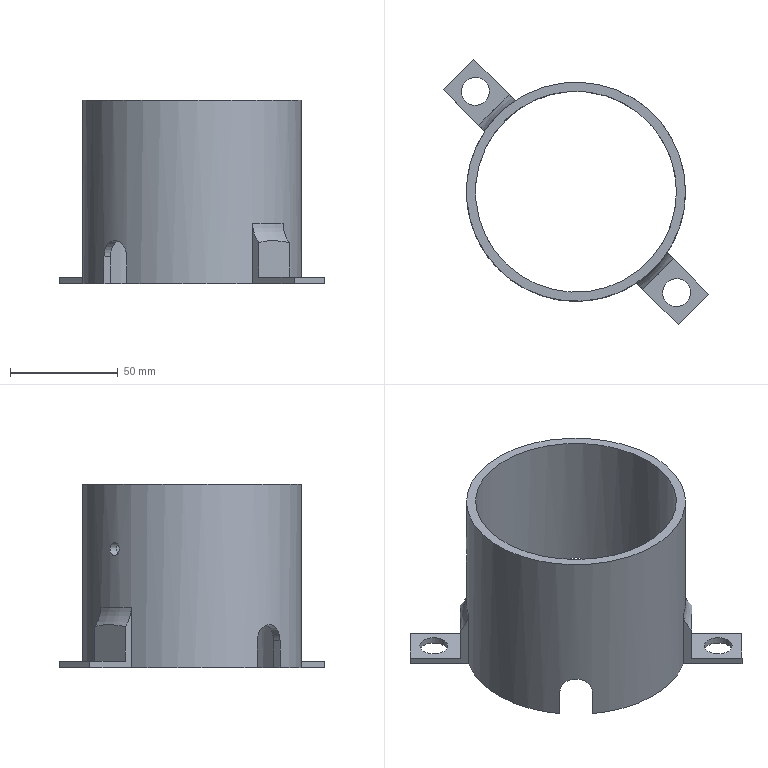Part | NX | features solid 2 | 1 solid | 26 faces | box 123.037 x 123.037 x 85 mm | volume 111745 mm3 | plane 17 | cylinder 7 | torus 2 | commonest cylinder face diameters 13 x2 15 x2 6 x1 93.2 x1 101.6 x1
STEP:
#1=CARTESIAN_POINT('',(-1552.073,-647.927,-105.));
#2=VERTEX_POINT('',#1);
#3=CARTESIAN_POINT('',(-1556.669,-643.331,-105.));
#4=DIRECTION('',(0.,0.,1.));
#5=DIRECTION('',(0.7071,-0.7071,0.));
#6=AXIS2_PLACEMENT_3D('',#3,#4,#5);
#7=CIRCLE('',#6,6.5);
#8=EDGE_CURVE('',#2,#2,#7,.T.);
#9=ORIENTED_EDGE('',*,*,#8,.T.);
#10=EDGE_LOOP('',(#9));
#11=FACE_BOUND('',#10,.T.);
#12=CARTESIAN_POINT('',(-1479.776,-649.169,-105.));
#13=VERTEX_POINT('',#12);
#14=CARTESIAN_POINT('',(-1538.147,-647.711,-105.));
#15=VERTEX_POINT('',#14);
#16=CARTESIAN_POINT('',(-1510.,-690.,-105.));
#17=DIRECTION('',(0.,0.,1.));
#18=DIRECTION('',(0.7071,-0.7071,0.));
#19=AXIS2_PLACEMENT_3D('',#16,#17,#18);
#20=CIRCLE('',#19,50.8);
#21=EDGE_CURVE('',#13,#15,#20,.T.);
#22=ORIENTED_EDGE('',*,*,#21,.F.);
#23=CARTESIAN_POINT('',(-1482.782,-652.175,-105.));
#24=VERTEX_POINT('',#23);
#25=CARTESIAN_POINT('',(-1515.303,-684.697,-105.));
#26=DIRECTION('',(-0.7071,-0.7071,0.));
#27=VECTOR('',#26,1000.);
#28=LINE('',#25,#27);
#29=EDGE_CURVE('',#13,#24,#28,.T.);
#30=ORIENTED_EDGE('',*,*,#29,.T.);
#31=CARTESIAN_POINT('',(-1547.825,-717.218,-105.));
#32=VERTEX_POINT('',#31);
#33=CARTESIAN_POINT('',(-1510.,-690.,-105.));
#34=DIRECTION('',(0.,0.,1.));
#35=DIRECTION('',(0.7071,-0.7071,0.));
#36=AXIS2_PLACEMENT_3D('',#33,#34,#35);
#37=CIRCLE('',#36,46.6);
#38=EDGE_CURVE('',#24,#32,#37,.T.);
#39=ORIENTED_EDGE('',*,*,#38,.T.);
#40=CARTESIAN_POINT('',(-1550.831,-720.224,-105.));
#41=VERTEX_POINT('',#40);
#42=CARTESIAN_POINT('',(-1515.303,-684.697,-105.));
#43=DIRECTION('',(-0.7071,-0.7071,0.));
#44=VECTOR('',#43,1000.);
#45=LINE('',#42,#44);
#46=EDGE_CURVE('',#32,#41,#45,.T.);
#47=ORIENTED_EDGE('',*,*,#46,.T.);
#48=CARTESIAN_POINT('',(-1552.289,-661.853,-105.));
#49=VERTEX_POINT('',#48);
#50=CARTESIAN_POINT('',(-1510.,-690.,-105.));
#51=DIRECTION('',(0.,0.,1.));
#52=DIRECTION('',(0.7071,-0.7071,0.));
#53=AXIS2_PLACEMENT_3D('',#50,#51,#52);
#54=CIRCLE('',#53,50.8);
#55=EDGE_CURVE('',#49,#41,#54,.T.);
#56=ORIENTED_EDGE('',*,*,#55,.F.);
#57=CARTESIAN_POINT('',(-1571.518,-642.624,-105.));
#58=VERTEX_POINT('',#57);
#59=CARTESIAN_POINT('',(-1561.619,-652.523,-105.));
#60=DIRECTION('',(0.7071,-0.7071,0.));
#61=VECTOR('',#60,1000.);
#62=LINE('',#59,#61);
#63=EDGE_CURVE('',#58,#49,#62,.T.);
#64=ORIENTED_EDGE('',*,*,#63,.F.);
#65=CARTESIAN_POINT('',(-1557.376,-628.482,-105.));
#66=VERTEX_POINT('',#65);
#67=CARTESIAN_POINT('',(-1571.518,-642.624,-105.));
#68=DIRECTION('',(0.7071,0.7071,0.));
#69=VECTOR('',#68,1000.);
#70=LINE('',#67,#69);
#71=EDGE_CURVE('',#58,#66,#70,.T.);
#72=ORIENTED_EDGE('',*,*,#71,.T.);
#73=CARTESIAN_POINT('',(-1541.113,-644.745,-105.));
#74=DIRECTION('',(-0.7071,0.7071,0.));
#75=VECTOR('',#74,1000.);
#76=LINE('',#73,#75);
#77=EDGE_CURVE('',#15,#66,#76,.T.);
#78=ORIENTED_EDGE('',*,*,#77,.F.);
#79=EDGE_LOOP('',(#22,#30,#39,#47,#56,#64,#72,#78));
#80=FACE_BOUND('',#79,.T.);
#81=CARTESIAN_POINT('',(-1510.,-690.,-105.));
#82=DIRECTION('',(0.,0.,1.));
#83=DIRECTION('',(0.7071,-0.7071,0.));
#84=AXIS2_PLACEMENT_3D('',#81,#82,#83);
#85=PLANE('',#84);
#86=ADVANCED_FACE('',(#11,#80),#85,.F.);
#87=CARTESIAN_POINT('',(-1546.112,-654.271,-52.988));
#88=VERTEX_POINT('',#87);
#89=CARTESIAN_POINT('',(-1547.688,-655.926,-52.127));
#90=CARTESIAN_POINT('',(-1546.147,-654.276,-53.312));
#91=CARTESIAN_POINT('',(-1544.392,-652.596,-52.552));
#92=CARTESIAN_POINT('',(-1543.503,-651.816,-50.302));
#93=CARTESIAN_POINT('',(-1544.075,-652.313,-47.871));
#94=CARTESIAN_POINT('',(-1545.724,-653.852,-46.689));
#95=CARTESIAN_POINT('',(-1547.402,-655.605,-47.445));
#96=CARTESIAN_POINT('',(-1548.185,-656.498,-49.697));
#97=CARTESIAN_POINT('',(-1547.688,-655.926,-52.127));
#98=CARTESIAN_POINT('',(-1546.147,-654.276,-53.312));
#99=CARTESIAN_POINT('',(-1544.392,-652.596,-52.552));
#100=B_SPLINE_CURVE_WITH_KNOTS('',3,(#89,#90,#91,#92,#93,#94,#95,#96,#97,#98,#99),.UNSPECIFIED.,.T.,.F.,(1,1,1,1,1,1,1,1,1,1,1,1,1,1,1),(-0.007035,-0.00469,-0.002345,0.,0.002345,0.00469,0.007035,0.00938,0.01173,0.01407,0.01642,0.01876,0.02111,0.02345,0.0258),.UNSPECIFIED.);
#101=EDGE_CURVE('',#88,#88,#100,.T.);
#102=ORIENTED_EDGE('',*,*,#101,.T.);
#103=EDGE_LOOP('',(#102));
#104=FACE_BOUND('',#103,.T.);
#105=CARTESIAN_POINT('',(-1459.2,-690.,-20.));
#106=VERTEX_POINT('',#105);
#107=CARTESIAN_POINT('',(-1510.,-690.,-20.));
#108=DIRECTION('',(0.,0.,1.));
#109=DIRECTION('',(1.,0.,0.));
#110=AXIS2_PLACEMENT_3D('',#107,#108,#109);
#111=CIRCLE('',#110,50.8);
#112=EDGE_CURVE('',#106,#106,#111,.T.);
#113=ORIENTED_EDGE('',*,*,#112,.F.);
#114=EDGE_LOOP('',(#113));
#115=FACE_BOUND('',#114,.T.);
#116=CARTESIAN_POINT('',(-1469.169,-659.776,-92.5));
#117=VERTEX_POINT('',#116);
#118=CARTESIAN_POINT('',(-1479.776,-649.169,-92.5));
#119=VERTEX_POINT('',#118);
#120=CARTESIAN_POINT('',(-1469.169,-659.776,-92.5));
#121=CARTESIAN_POINT('',(-1469.169,-659.776,-90.54));
#122=CARTESIAN_POINT('',(-1470.113,-658.437,-86.63));
#123=CARTESIAN_POINT('',(-1473.989,-653.973,-84.184));
#124=CARTESIAN_POINT('',(-1478.43,-650.12,-86.635));
#125=CARTESIAN_POINT('',(-1479.776,-649.169,-90.52));
#126=CARTESIAN_POINT('',(-1479.776,-649.169,-92.5));
#127=B_SPLINE_CURVE_WITH_KNOTS('',3,(#120,#121,#122,#123,#124,#125,#126),.UNSPECIFIED.,.F.,.F.,(4,1,1,1,4),(0.03594,0.04181,0.04767,0.05354,0.05941),.UNSPECIFIED.);
#128=EDGE_CURVE('',#117,#119,#127,.T.);
#129=ORIENTED_EDGE('',*,*,#128,.T.);
#130=CARTESIAN_POINT('',(-1479.776,-649.169,5.));
#131=DIRECTION('',(0.,0.,-1.));
#132=VECTOR('',#131,1000.);
#133=LINE('',#130,#132);
#134=EDGE_CURVE('',#119,#13,#133,.T.);
#135=ORIENTED_EDGE('',*,*,#134,.T.);
#136=ORIENTED_EDGE('',*,*,#21,.T.);
#137=CARTESIAN_POINT('',(-1538.147,-647.711,-77.));
#138=VERTEX_POINT('',#137);
#139=CARTESIAN_POINT('',(-1538.147,-647.711,5.));
#140=DIRECTION('',(0.,0.,-1.));
#141=VECTOR('',#140,1000.);
#142=LINE('',#139,#141);
#143=EDGE_CURVE('',#138,#15,#142,.T.);
#144=ORIENTED_EDGE('',*,*,#143,.F.);
#145=CARTESIAN_POINT('',(-1552.289,-661.853,-77.));
#146=VERTEX_POINT('',#145);
#147=CARTESIAN_POINT('',(-1510.,-690.,-77.));
#148=DIRECTION('',(0.,0.,-1.));
#149=DIRECTION('',(-0.7071,0.7071,0.));
#150=AXIS2_PLACEMENT_3D('',#147,#148,#149);
#151=CIRCLE('',#150,50.8);
#152=EDGE_CURVE('',#138,#146,#151,.F.);
#153=ORIENTED_EDGE('',*,*,#152,.T.);
#154=CARTESIAN_POINT('',(-1552.289,-661.853,-105.));
#155=DIRECTION('',(0.,0.,-1.));
#156=VECTOR('',#155,1000.);
#157=LINE('',#154,#156);
#158=EDGE_CURVE('',#49,#146,#157,.F.);
#159=ORIENTED_EDGE('',*,*,#158,.F.);
#160=ORIENTED_EDGE('',*,*,#55,.T.);
#161=CARTESIAN_POINT('',(-1550.831,-720.224,-92.5));
#162=VERTEX_POINT('',#161);
#163=CARTESIAN_POINT('',(-1550.831,-720.224,5.));
#164=DIRECTION('',(0.,0.,-1.));
#165=VECTOR('',#164,1000.);
#166=LINE('',#163,#165);
#167=EDGE_CURVE('',#41,#162,#166,.F.);
#168=ORIENTED_EDGE('',*,*,#167,.T.);
#169=CARTESIAN_POINT('',(-1540.224,-730.831,-92.5));
#170=VERTEX_POINT('',#169);
#171=CARTESIAN_POINT('',(-1550.831,-720.224,-92.5));
#172=CARTESIAN_POINT('',(-1550.831,-720.224,-90.517));
#173=CARTESIAN_POINT('',(-1549.882,-721.568,-86.634));
#174=CARTESIAN_POINT('',(-1546.014,-726.024,-84.184));
#175=CARTESIAN_POINT('',(-1541.566,-729.884,-86.631));
#176=CARTESIAN_POINT('',(-1540.224,-730.831,-90.541));
#177=CARTESIAN_POINT('',(-1540.224,-730.831,-92.5));
#178=B_SPLINE_CURVE_WITH_KNOTS('',3,(#171,#172,#173,#174,#175,#176,#177),.UNSPECIFIED.,.F.,.F.,(4,1,1,1,4),(0.03522,0.04109,0.04696,0.05283,0.0587),.UNSPECIFIED.);
#179=EDGE_CURVE('',#162,#170,#178,.T.);
#180=ORIENTED_EDGE('',*,*,#179,.T.);
#181=CARTESIAN_POINT('',(-1540.224,-730.831,-105.));
#182=VERTEX_POINT('',#181);
#183=CARTESIAN_POINT('',(-1540.224,-730.831,5.));
#184=DIRECTION('',(0.,0.,-1.));
#185=VECTOR('',#184,1000.);
#186=LINE('',#183,#185);
#187=EDGE_CURVE('',#170,#182,#186,.T.);
#188=ORIENTED_EDGE('',*,*,#187,.T.);
#189=CARTESIAN_POINT('',(-1481.853,-732.289,-105.));
#190=VERTEX_POINT('',#189);
#191=CARTESIAN_POINT('',(-1510.,-690.,-105.));
#192=DIRECTION('',(0.,0.,1.));
#193=DIRECTION('',(0.7071,-0.7071,0.));
#194=AXIS2_PLACEMENT_3D('',#191,#192,#193);
#195=CIRCLE('',#194,50.8);
#196=EDGE_CURVE('',#182,#190,#195,.T.);
#197=ORIENTED_EDGE('',*,*,#196,.T.);
#198=CARTESIAN_POINT('',(-1481.853,-732.289,-77.));
#199=VERTEX_POINT('',#198);
#200=CARTESIAN_POINT('',(-1481.853,-732.289,5.));
#201=DIRECTION('',(0.,0.,-1.));
#202=VECTOR('',#201,1000.);
#203=LINE('',#200,#202);
#204=EDGE_CURVE('',#199,#190,#203,.T.);
#205=ORIENTED_EDGE('',*,*,#204,.F.);
#206=CARTESIAN_POINT('',(-1467.711,-718.147,-77.));
#207=VERTEX_POINT('',#206);
#208=CARTESIAN_POINT('',(-1510.,-690.,-77.));
#209=DIRECTION('',(0.,0.,-1.));
#210=DIRECTION('',(-0.7071,0.7071,0.));
#211=AXIS2_PLACEMENT_3D('',#208,#209,#210);
#212=CIRCLE('',#211,50.8);
#213=EDGE_CURVE('',#199,#207,#212,.F.);
#214=ORIENTED_EDGE('',*,*,#213,.T.);
#215=CARTESIAN_POINT('',(-1467.711,-718.147,-105.));
#216=VERTEX_POINT('',#215);
#217=CARTESIAN_POINT('',(-1467.711,-718.147,-105.));
#218=DIRECTION('',(0.,0.,-1.));
#219=VECTOR('',#218,1000.);
#220=LINE('',#217,#219);
#221=EDGE_CURVE('',#216,#207,#220,.F.);
#222=ORIENTED_EDGE('',*,*,#221,.F.);
#223=CARTESIAN_POINT('',(-1469.169,-659.776,-105.));
#224=VERTEX_POINT('',#223);
#225=CARTESIAN_POINT('',(-1510.,-690.,-105.));
#226=DIRECTION('',(0.,0.,1.));
#227=DIRECTION('',(0.7071,-0.7071,0.));
#228=AXIS2_PLACEMENT_3D('',#225,#226,#227);
#229=CIRCLE('',#228,50.8);
#230=EDGE_CURVE('',#216,#224,#229,.T.);
#231=ORIENTED_EDGE('',*,*,#230,.T.);
#232=CARTESIAN_POINT('',(-1469.169,-659.776,5.));
#233=DIRECTION('',(0.,0.,-1.));
#234=VECTOR('',#233,1000.);
#235=LINE('',#232,#234);
#236=EDGE_CURVE('',#224,#117,#235,.F.);
#237=ORIENTED_EDGE('',*,*,#236,.T.);
#238=EDGE_LOOP('',(#129,#135,#136,#144,#153,#159,#160,#168,#180,#188,#197,#205,#214,#222,#231,#237));
#239=FACE_BOUND('',#238,.T.);
#240=CARTESIAN_POINT('',(-1510.,-690.,5.));
#241=DIRECTION('',(0.,0.,-1.));
#242=DIRECTION('',(-0.7071,0.7071,0.));
#243=AXIS2_PLACEMENT_3D('',#240,#241,#242);
#244=CYLINDRICAL_SURFACE('',#243,50.8);
#245=ADVANCED_FACE('',(#104,#115,#239),#244,.T.);
#246=CARTESIAN_POINT('',(-1482.782,-652.175,-92.5));
#247=VERTEX_POINT('',#246);
#248=CARTESIAN_POINT('',(-1482.782,-652.175,5.));
#249=DIRECTION('',(0.,0.,-1.));
#250=VECTOR('',#249,1000.);
#251=LINE('',#248,#250);
#252=EDGE_CURVE('',#247,#24,#251,.T.);
#253=ORIENTED_EDGE('',*,*,#252,.F.);
#254=CARTESIAN_POINT('',(-1472.175,-662.782,-92.5));
#255=VERTEX_POINT('',#254);
#256=CARTESIAN_POINT('',(-1472.175,-662.782,-92.5));
#257=CARTESIAN_POINT('',(-1472.175,-662.782,-90.515));
#258=CARTESIAN_POINT('',(-1473.108,-661.416,-86.635));
#259=CARTESIAN_POINT('',(-1476.936,-656.948,-84.184));
#260=CARTESIAN_POINT('',(-1481.415,-653.108,-86.63));
#261=CARTESIAN_POINT('',(-1482.782,-652.175,-90.515));
#262=CARTESIAN_POINT('',(-1482.782,-652.175,-92.5));
#263=B_SPLINE_CURVE_WITH_KNOTS('',3,(#256,#257,#258,#259,#260,#261,#262),.UNSPECIFIED.,.F.,.F.,(4,1,1,1,4),(0.,0.00587,0.01174,0.01761,0.02348),.UNSPECIFIED.);
#264=EDGE_CURVE('',#255,#247,#263,.T.);
#265=ORIENTED_EDGE('',*,*,#264,.F.);
#266=CARTESIAN_POINT('',(-1472.175,-662.782,-105.));
#267=VERTEX_POINT('',#266);
#268=CARTESIAN_POINT('',(-1472.175,-662.782,5.));
#269=DIRECTION('',(0.,0.,-1.));
#270=VECTOR('',#269,1000.);
#271=LINE('',#268,#270);
#272=EDGE_CURVE('',#267,#255,#271,.F.);
#273=ORIENTED_EDGE('',*,*,#272,.F.);
#274=CARTESIAN_POINT('',(-1537.218,-727.825,-105.));
#275=VERTEX_POINT('',#274);
#276=CARTESIAN_POINT('',(-1510.,-690.,-105.));
#277=DIRECTION('',(0.,0.,1.));
#278=DIRECTION('',(0.7071,-0.7071,0.));
#279=AXIS2_PLACEMENT_3D('',#276,#277,#278);
#280=CIRCLE('',#279,46.6);
#281=EDGE_CURVE('',#275,#267,#280,.T.);
#282=ORIENTED_EDGE('',*,*,#281,.F.);
#283=CARTESIAN_POINT('',(-1537.218,-727.825,-92.5));
#284=VERTEX_POINT('',#283);
#285=CARTESIAN_POINT('',(-1537.218,-727.825,5.));
#286=DIRECTION('',(0.,0.,-1.));
#287=VECTOR('',#286,1000.);
#288=LINE('',#285,#287);
#289=EDGE_CURVE('',#284,#275,#288,.T.);
#290=ORIENTED_EDGE('',*,*,#289,.F.);
#291=CARTESIAN_POINT('',(-1547.825,-717.218,-92.5));
#292=VERTEX_POINT('',#291);
#293=CARTESIAN_POINT('',(-1547.825,-717.218,-92.5));
#294=CARTESIAN_POINT('',(-1547.825,-717.218,-90.518));
#295=CARTESIAN_POINT('',(-1546.895,-718.58,-86.634));
#296=CARTESIAN_POINT('',(-1543.053,-723.063,-84.183));
#297=CARTESIAN_POINT('',(-1538.578,-726.896,-86.632));
#298=CARTESIAN_POINT('',(-1537.218,-727.825,-90.54));
#299=CARTESIAN_POINT('',(-1537.218,-727.825,-92.5));
#300=B_SPLINE_CURVE_WITH_KNOTS('',3,(#293,#294,#295,#296,#297,#298,#299),.UNSPECIFIED.,.F.,.F.,(4,1,1,1,4),(0.03523,0.0411,0.04697,0.05284,0.05871),.UNSPECIFIED.);
#301=EDGE_CURVE('',#292,#284,#300,.T.);
#302=ORIENTED_EDGE('',*,*,#301,.F.);
#303=CARTESIAN_POINT('',(-1547.825,-717.218,5.));
#304=DIRECTION('',(0.,0.,-1.));
#305=VECTOR('',#304,1000.);
#306=LINE('',#303,#305);
#307=EDGE_CURVE('',#32,#292,#306,.F.);
#308=ORIENTED_EDGE('',*,*,#307,.F.);
#309=ORIENTED_EDGE('',*,*,#38,.F.);
#310=EDGE_LOOP('',(#253,#265,#273,#282,#290,#302,#308,#309));
#311=FACE_BOUND('',#310,.T.);
#312=CARTESIAN_POINT('',(-1543.146,-657.245,-52.987));
#313=VERTEX_POINT('',#312);
#314=CARTESIAN_POINT('',(-1544.717,-658.902,-52.122));
#315=CARTESIAN_POINT('',(-1543.184,-657.249,-53.311));
#316=CARTESIAN_POINT('',(-1541.424,-655.571,-52.556));
#317=CARTESIAN_POINT('',(-1540.526,-654.793,-50.309));
#318=CARTESIAN_POINT('',(-1541.098,-655.283,-47.876));
#319=CARTESIAN_POINT('',(-1542.751,-656.816,-46.69));
#320=CARTESIAN_POINT('',(-1544.427,-658.574,-47.441));
#321=CARTESIAN_POINT('',(-1545.207,-659.474,-49.69));
#322=CARTESIAN_POINT('',(-1544.717,-658.902,-52.122));
#323=CARTESIAN_POINT('',(-1543.184,-657.249,-53.311));
#324=CARTESIAN_POINT('',(-1541.424,-655.571,-52.556));
#325=B_SPLINE_CURVE_WITH_KNOTS('',3,(#314,#315,#316,#317,#318,#319,#320,#321,#322,#323,#324),.UNSPECIFIED.,.T.,.F.,(1,1,1,1,1,1,1,1,1,1,1,1,1,1,1),(-0.007036,-0.00469,-0.002345,0.,0.002345,0.00469,0.007036,0.009381,0.01173,0.01407,0.01642,0.01876,0.02111,0.02345,0.0258),.UNSPECIFIED.);
#326=EDGE_CURVE('',#313,#313,#325,.T.);
#327=ORIENTED_EDGE('',*,*,#326,.F.);
#328=EDGE_LOOP('',(#327));
#329=FACE_BOUND('',#328,.T.);
#330=CARTESIAN_POINT('',(-1463.4,-690.,-20.));
#331=VERTEX_POINT('',#330);
#332=CARTESIAN_POINT('',(-1510.,-690.,-20.));
#333=DIRECTION('',(0.,0.,1.));
#334=DIRECTION('',(1.,0.,0.));
#335=AXIS2_PLACEMENT_3D('',#332,#333,#334);
#336=CIRCLE('',#335,46.6);
#337=EDGE_CURVE('',#331,#331,#336,.T.);
#338=ORIENTED_EDGE('',*,*,#337,.T.);
#339=EDGE_LOOP('',(#338));
#340=FACE_BOUND('',#339,.T.);
#341=CARTESIAN_POINT('',(-1510.,-690.,5.));
#342=DIRECTION('',(0.,0.,-1.));
#343=DIRECTION('',(-0.7071,0.7071,0.));
#344=AXIS2_PLACEMENT_3D('',#341,#342,#343);
#345=CYLINDRICAL_SURFACE('',#344,46.6);
#346=ADVANCED_FACE('',(#311,#329,#340),#345,.F.);
#347=ORIENTED_EDGE('',*,*,#337,.F.);
#348=EDGE_LOOP('',(#347));
#349=FACE_BOUND('',#348,.T.);
#350=ORIENTED_EDGE('',*,*,#112,.T.);
#351=EDGE_LOOP('',(#350));
#352=FACE_BOUND('',#351,.T.);
#353=CARTESIAN_POINT('',(-1510.,-690.,-20.));
#354=DIRECTION('',(0.,0.,1.));
#355=DIRECTION('',(0.7071,-0.7071,0.));
#356=AXIS2_PLACEMENT_3D('',#353,#354,#355);
#357=PLANE('',#356);
#358=ADVANCED_FACE('',(#349,#352),#357,.T.);
#359=ORIENTED_EDGE('',*,*,#281,.T.);
#360=CARTESIAN_POINT('',(-1504.697,-695.303,-105.));
#361=DIRECTION('',(0.7071,0.7071,0.));
#362=VECTOR('',#361,1000.);
#363=LINE('',#360,#362);
#364=EDGE_CURVE('',#267,#224,#363,.T.);
#365=ORIENTED_EDGE('',*,*,#364,.T.);
#366=ORIENTED_EDGE('',*,*,#230,.F.);
#367=CARTESIAN_POINT('',(-1448.482,-737.376,-105.));
#368=VERTEX_POINT('',#367);
#369=CARTESIAN_POINT('',(-1458.381,-727.477,-105.));
#370=DIRECTION('',(-0.7071,0.7071,0.));
#371=VECTOR('',#370,1000.);
#372=LINE('',#369,#371);
#373=EDGE_CURVE('',#368,#216,#372,.T.);
#374=ORIENTED_EDGE('',*,*,#373,.F.);
#375=CARTESIAN_POINT('',(-1462.624,-751.518,-105.));
#376=VERTEX_POINT('',#375);
#377=CARTESIAN_POINT('',(-1448.482,-737.376,-105.));
#378=DIRECTION('',(-0.7071,-0.7071,0.));
#379=VECTOR('',#378,1000.);
#380=LINE('',#377,#379);
#381=EDGE_CURVE('',#368,#376,#380,.T.);
#382=ORIENTED_EDGE('',*,*,#381,.T.);
#383=CARTESIAN_POINT('',(-1478.887,-735.255,-105.));
#384=DIRECTION('',(0.7071,-0.7071,0.));
#385=VECTOR('',#384,1000.);
#386=LINE('',#383,#385);
#387=EDGE_CURVE('',#190,#376,#386,.T.);
#388=ORIENTED_EDGE('',*,*,#387,.F.);
#389=ORIENTED_EDGE('',*,*,#196,.F.);
#390=CARTESIAN_POINT('',(-1504.697,-695.303,-105.));
#391=DIRECTION('',(0.7071,0.7071,0.));
#392=VECTOR('',#391,1000.);
#393=LINE('',#390,#392);
#394=EDGE_CURVE('',#182,#275,#393,.T.);
#395=ORIENTED_EDGE('',*,*,#394,.T.);
#396=EDGE_LOOP('',(#359,#365,#366,#374,#382,#388,#389,#395));
#397=FACE_BOUND('',#396,.T.);
#398=CARTESIAN_POINT('',(-1458.735,-741.265,-105.));
#399=VERTEX_POINT('',#398);
#400=CARTESIAN_POINT('',(-1463.331,-736.669,-105.));
#401=DIRECTION('',(0.,0.,1.));
#402=DIRECTION('',(0.7071,-0.7071,0.));
#403=AXIS2_PLACEMENT_3D('',#400,#401,#402);
#404=CIRCLE('',#403,6.5);
#405=EDGE_CURVE('',#399,#399,#404,.T.);
#406=ORIENTED_EDGE('',*,*,#405,.T.);
#407=EDGE_LOOP('',(#406));
#408=FACE_BOUND('',#407,.T.);
#409=CARTESIAN_POINT('',(-1510.,-690.,-105.));
#410=DIRECTION('',(0.,0.,1.));
#411=DIRECTION('',(0.7071,-0.7071,0.));
#412=AXIS2_PLACEMENT_3D('',#409,#410,#411);
#413=PLANE('',#412);
#414=ADVANCED_FACE('',(#397,#408),#413,.F.);
#415=ORIENTED_EDGE('',*,*,#63,.T.);
#416=ORIENTED_EDGE('',*,*,#158,.T.);
#417=CARTESIAN_POINT('',(-1555.113,-659.029,-85.961));
#418=VERTEX_POINT('',#417);
#419=CARTESIAN_POINT('',(-1552.289,-661.853,-77.));
#420=CARTESIAN_POINT('',(-1552.289,-661.853,-80.399));
#421=CARTESIAN_POINT('',(-1553.359,-660.783,-83.708));
#422=CARTESIAN_POINT('',(-1555.113,-659.029,-85.961));
#423=B_SPLINE_CURVE_WITH_KNOTS('',3,(#419,#420,#421,#422),.UNSPECIFIED.,.F.,.F.,(4,4),(0.,0.01005),.UNSPECIFIED.);
#424=EDGE_CURVE('',#146,#418,#423,.T.);
#425=ORIENTED_EDGE('',*,*,#424,.T.);
#426=CARTESIAN_POINT('',(-1555.113,-659.029,-102.));
#427=VERTEX_POINT('',#426);
#428=CARTESIAN_POINT('',(-1555.113,-659.029,-80.));
#429=DIRECTION('',(0.,0.,-1.));
#430=VECTOR('',#429,1000.);
#431=LINE('',#428,#430);
#432=EDGE_CURVE('',#418,#427,#431,.T.);
#433=ORIENTED_EDGE('',*,*,#432,.T.);
#434=CARTESIAN_POINT('',(-1571.518,-642.624,-102.));
#435=VERTEX_POINT('',#434);
#436=CARTESIAN_POINT('',(-1561.619,-652.523,-102.));
#437=DIRECTION('',(-0.7071,0.7071,0.));
#438=VECTOR('',#437,1000.);
#439=LINE('',#436,#438);
#440=EDGE_CURVE('',#427,#435,#439,.T.);
#441=ORIENTED_EDGE('',*,*,#440,.T.);
#442=CARTESIAN_POINT('',(-1571.518,-642.624,-102.));
#443=DIRECTION('',(0.,0.,-1.));
#444=VECTOR('',#443,1000.);
#445=LINE('',#442,#444);
#446=EDGE_CURVE('',#435,#58,#445,.T.);
#447=ORIENTED_EDGE('',*,*,#446,.T.);
#448=EDGE_LOOP('',(#415,#416,#425,#433,#441,#447));
#449=FACE_BOUND('',#448,.T.);
#450=CARTESIAN_POINT('',(-1561.619,-652.523,-80.));
#451=DIRECTION('',(0.7071,0.7071,0.));
#452=DIRECTION('',(-0.7071,0.7071,0.));
#453=AXIS2_PLACEMENT_3D('',#450,#451,#452);
#454=PLANE('',#453);
#455=ADVANCED_FACE('',(#449),#454,.F.);
#456=CARTESIAN_POINT('',(-1540.971,-644.887,-85.961));
#457=VERTEX_POINT('',#456);
#458=CARTESIAN_POINT('',(-1540.971,-644.887,-102.));
#459=VERTEX_POINT('',#458);
#460=CARTESIAN_POINT('',(-1540.971,-644.887,-80.));
#461=DIRECTION('',(0.,0.,-1.));
#462=VECTOR('',#461,1000.);
#463=LINE('',#460,#462);
#464=EDGE_CURVE('',#457,#459,#463,.T.);
#465=ORIENTED_EDGE('',*,*,#464,.F.);
#466=CARTESIAN_POINT('',(-1540.971,-644.887,-85.961));
#467=CARTESIAN_POINT('',(-1539.209,-646.649,-83.698));
#468=CARTESIAN_POINT('',(-1538.147,-647.711,-80.397));
#469=CARTESIAN_POINT('',(-1538.147,-647.711,-77.));
#470=B_SPLINE_CURVE_WITH_KNOTS('',3,(#466,#467,#468,#469),.UNSPECIFIED.,.F.,.F.,(4,4),(0.009164,0.01921),.UNSPECIFIED.);
#471=EDGE_CURVE('',#457,#138,#470,.T.);
#472=ORIENTED_EDGE('',*,*,#471,.T.);
#473=ORIENTED_EDGE('',*,*,#143,.T.);
#474=ORIENTED_EDGE('',*,*,#77,.T.);
#475=CARTESIAN_POINT('',(-1557.376,-628.482,-102.));
#476=VERTEX_POINT('',#475);
#477=CARTESIAN_POINT('',(-1557.376,-628.482,-102.));
#478=DIRECTION('',(0.,0.,-1.));
#479=VECTOR('',#478,1000.);
#480=LINE('',#477,#479);
#481=EDGE_CURVE('',#476,#66,#480,.T.);
#482=ORIENTED_EDGE('',*,*,#481,.F.);
#483=CARTESIAN_POINT('',(-1563.033,-622.825,-102.));
#484=DIRECTION('',(0.7071,-0.7071,0.));
#485=VECTOR('',#484,1000.);
#486=LINE('',#483,#485);
#487=EDGE_CURVE('',#476,#459,#486,.T.);
#488=ORIENTED_EDGE('',*,*,#487,.T.);
#489=EDGE_LOOP('',(#465,#472,#473,#474,#482,#488));
#490=FACE_BOUND('',#489,.T.);
#491=CARTESIAN_POINT('',(-1541.113,-644.745,-80.));
#492=DIRECTION('',(-0.7071,-0.7071,0.));
#493=DIRECTION('',(0.7071,-0.7071,0.));
#494=AXIS2_PLACEMENT_3D('',#491,#492,#493);
#495=PLANE('',#494);
#496=ADVANCED_FACE('',(#490),#495,.F.);
#497=ORIENTED_EDGE('',*,*,#464,.T.);
#498=CARTESIAN_POINT('',(-1540.971,-644.887,-102.));
#499=DIRECTION('',(-0.7071,-0.7071,0.));
#500=VECTOR('',#499,1000.);
#501=LINE('',#498,#500);
#502=EDGE_CURVE('',#459,#427,#501,.T.);
#503=ORIENTED_EDGE('',*,*,#502,.T.);
#504=ORIENTED_EDGE('',*,*,#432,.F.);
#505=CARTESIAN_POINT('',(-1555.113,-659.029,-85.961));
#506=CARTESIAN_POINT('',(-1552.787,-656.702,-85.406));
#507=CARTESIAN_POINT('',(-1549.281,-653.196,-84.828));
#508=CARTESIAN_POINT('',(-1545.145,-649.06,-85.143));
#509=CARTESIAN_POINT('',(-1543.054,-646.969,-85.504));
#510=CARTESIAN_POINT('',(-1541.876,-645.791,-85.751));
#511=CARTESIAN_POINT('',(-1541.25,-645.165,-85.895));
#512=CARTESIAN_POINT('',(-1540.971,-644.887,-85.961));
#513=B_SPLINE_CURVE_WITH_KNOTS('',3,(#505,#506,#507,#508,#509,#510,#511,#512),.UNSPECIFIED.,.F.,.F.,(4,1,1,1,1,4),(0.21,0.2196,0.2244,0.2268,0.228,0.2292),.UNSPECIFIED.);
#514=EDGE_CURVE('',#457,#418,#513,.F.);
#515=ORIENTED_EDGE('',*,*,#514,.F.);
#516=EDGE_LOOP('',(#497,#503,#504,#515));
#517=FACE_BOUND('',#516,.T.);
#518=CARTESIAN_POINT('',(-1540.971,-644.887,-80.));
#519=DIRECTION('',(0.7071,-0.7071,0.));
#520=DIRECTION('',(0.,0.,-1.));
#521=AXIS2_PLACEMENT_3D('',#518,#519,#520);
#522=PLANE('',#521);
#523=ADVANCED_FACE('',(#517),#522,.F.);
#524=ORIENTED_EDGE('',*,*,#373,.T.);
#525=ORIENTED_EDGE('',*,*,#221,.T.);
#526=CARTESIAN_POINT('',(-1464.887,-720.971,-85.961));
#527=VERTEX_POINT('',#526);
#528=CARTESIAN_POINT('',(-1467.711,-718.147,-77.));
#529=CARTESIAN_POINT('',(-1467.711,-718.147,-80.399));
#530=CARTESIAN_POINT('',(-1466.641,-719.217,-83.708));
#531=CARTESIAN_POINT('',(-1464.887,-720.971,-85.961));
#532=B_SPLINE_CURVE_WITH_KNOTS('',3,(#528,#529,#530,#531),.UNSPECIFIED.,.F.,.F.,(4,4),(0.,0.01005),.UNSPECIFIED.);
#533=EDGE_CURVE('',#207,#527,#532,.T.);
#534=ORIENTED_EDGE('',*,*,#533,.T.);
#535=CARTESIAN_POINT('',(-1464.887,-720.971,-102.));
#536=VERTEX_POINT('',#535);
#537=CARTESIAN_POINT('',(-1464.887,-720.971,-80.));
#538=DIRECTION('',(0.,0.,-1.));
#539=VECTOR('',#538,1000.);
#540=LINE('',#537,#539);
#541=EDGE_CURVE('',#527,#536,#540,.T.);
#542=ORIENTED_EDGE('',*,*,#541,.T.);
#543=CARTESIAN_POINT('',(-1448.482,-737.376,-102.));
#544=VERTEX_POINT('',#543);
#545=CARTESIAN_POINT('',(-1458.381,-727.477,-102.));
#546=DIRECTION('',(0.7071,-0.7071,0.));
#547=VECTOR('',#546,1000.);
#548=LINE('',#545,#547);
#549=EDGE_CURVE('',#536,#544,#548,.T.);
#550=ORIENTED_EDGE('',*,*,#549,.T.);
#551=CARTESIAN_POINT('',(-1448.482,-737.376,-102.));
#552=DIRECTION('',(0.,0.,-1.));
#553=VECTOR('',#552,1000.);
#554=LINE('',#551,#553);
#555=EDGE_CURVE('',#544,#368,#554,.T.);
#556=ORIENTED_EDGE('',*,*,#555,.T.);
#557=EDGE_LOOP('',(#524,#525,#534,#542,#550,#556));
#558=FACE_BOUND('',#557,.T.);
#559=CARTESIAN_POINT('',(-1458.381,-727.477,-80.));
#560=DIRECTION('',(-0.7071,-0.7071,0.));
#561=DIRECTION('',(0.7071,-0.7071,0.));
#562=AXIS2_PLACEMENT_3D('',#559,#560,#561);
#563=PLANE('',#562);
#564=ADVANCED_FACE('',(#558),#563,.F.);
#565=CARTESIAN_POINT('',(-1479.029,-735.113,-85.961));
#566=VERTEX_POINT('',#565);
#567=CARTESIAN_POINT('',(-1479.029,-735.113,-102.));
#568=VERTEX_POINT('',#567);
#569=CARTESIAN_POINT('',(-1479.029,-735.113,-80.));
#570=DIRECTION('',(0.,0.,-1.));
#571=VECTOR('',#570,1000.);
#572=LINE('',#569,#571);
#573=EDGE_CURVE('',#566,#568,#572,.T.);
#574=ORIENTED_EDGE('',*,*,#573,.F.);
#575=CARTESIAN_POINT('',(-1479.029,-735.113,-85.961));
#576=CARTESIAN_POINT('',(-1480.791,-733.351,-83.698));
#577=CARTESIAN_POINT('',(-1481.853,-732.289,-80.397));
#578=CARTESIAN_POINT('',(-1481.853,-732.289,-77.));
#579=B_SPLINE_CURVE_WITH_KNOTS('',3,(#575,#576,#577,#578),.UNSPECIFIED.,.F.,.F.,(4,4),(0.009164,0.01921),.UNSPECIFIED.);
#580=EDGE_CURVE('',#566,#199,#579,.T.);
#581=ORIENTED_EDGE('',*,*,#580,.T.);
#582=ORIENTED_EDGE('',*,*,#204,.T.);
#583=ORIENTED_EDGE('',*,*,#387,.T.);
#584=CARTESIAN_POINT('',(-1462.624,-751.518,-102.));
#585=VERTEX_POINT('',#584);
#586=CARTESIAN_POINT('',(-1462.624,-751.518,-102.));
#587=DIRECTION('',(0.,0.,-1.));
#588=VECTOR('',#587,1000.);
#589=LINE('',#586,#588);
#590=EDGE_CURVE('',#585,#376,#589,.T.);
#591=ORIENTED_EDGE('',*,*,#590,.F.);
#592=CARTESIAN_POINT('',(-1456.967,-757.175,-102.));
#593=DIRECTION('',(-0.7071,0.7071,0.));
#594=VECTOR('',#593,1000.);
#595=LINE('',#592,#594);
#596=EDGE_CURVE('',#585,#568,#595,.T.);
#597=ORIENTED_EDGE('',*,*,#596,.T.);
#598=EDGE_LOOP('',(#574,#581,#582,#583,#591,#597));
#599=FACE_BOUND('',#598,.T.);
#600=CARTESIAN_POINT('',(-1478.887,-735.255,-80.));
#601=DIRECTION('',(0.7071,0.7071,0.));
#602=DIRECTION('',(0.,0.,1.));
#603=AXIS2_PLACEMENT_3D('',#600,#601,#602);
#604=PLANE('',#603);
#605=ADVANCED_FACE('',(#599),#604,.F.);
#606=ORIENTED_EDGE('',*,*,#573,.T.);
#607=CARTESIAN_POINT('',(-1479.029,-735.113,-102.));
#608=DIRECTION('',(0.7071,0.7071,0.));
#609=VECTOR('',#608,1000.);
#610=LINE('',#607,#609);
#611=EDGE_CURVE('',#568,#536,#610,.T.);
#612=ORIENTED_EDGE('',*,*,#611,.T.);
#613=ORIENTED_EDGE('',*,*,#541,.F.);
#614=CARTESIAN_POINT('',(-1464.887,-720.971,-85.961));
#615=CARTESIAN_POINT('',(-1467.213,-723.298,-85.406));
#616=CARTESIAN_POINT('',(-1470.719,-726.804,-84.828));
#617=CARTESIAN_POINT('',(-1474.855,-730.94,-85.143));
#618=CARTESIAN_POINT('',(-1476.946,-733.031,-85.504));
#619=CARTESIAN_POINT('',(-1478.124,-734.209,-85.751));
#620=CARTESIAN_POINT('',(-1478.75,-734.835,-85.895));
#621=CARTESIAN_POINT('',(-1479.029,-735.113,-85.961));
#622=B_SPLINE_CURVE_WITH_KNOTS('',3,(#614,#615,#616,#617,#618,#619,#620,#621),.UNSPECIFIED.,.F.,.F.,(4,1,1,1,1,4),(0.21,0.2196,0.2244,0.2268,0.228,0.2292),.UNSPECIFIED.);
#623=EDGE_CURVE('',#566,#527,#622,.F.);
#624=ORIENTED_EDGE('',*,*,#623,.F.);
#625=EDGE_LOOP('',(#606,#612,#613,#624));
#626=FACE_BOUND('',#625,.T.);
#627=CARTESIAN_POINT('',(-1479.029,-735.113,-80.));
#628=DIRECTION('',(-0.7071,0.7071,0.));
#629=DIRECTION('',(0.,0.,1.));
#630=AXIS2_PLACEMENT_3D('',#627,#628,#629);
#631=PLANE('',#630);
#632=ADVANCED_FACE('',(#626),#631,.F.);
#633=ORIENTED_EDGE('',*,*,#381,.F.);
#634=ORIENTED_EDGE('',*,*,#555,.F.);
#635=CARTESIAN_POINT('',(-1448.482,-737.376,-102.));
#636=DIRECTION('',(-0.7071,-0.7071,0.));
#637=VECTOR('',#636,1000.);
#638=LINE('',#635,#637);
#639=EDGE_CURVE('',#544,#585,#638,.T.);
#640=ORIENTED_EDGE('',*,*,#639,.T.);
#641=ORIENTED_EDGE('',*,*,#590,.T.);
#642=EDGE_LOOP('',(#633,#634,#640,#641));
#643=FACE_BOUND('',#642,.T.);
#644=CARTESIAN_POINT('',(-1448.482,-737.376,-102.));
#645=DIRECTION('',(0.7071,-0.7071,0.));
#646=DIRECTION('',(0.,0.,-1.));
#647=AXIS2_PLACEMENT_3D('',#644,#645,#646);
#648=PLANE('',#647);
#649=ADVANCED_FACE('',(#643),#648,.T.);
#650=CARTESIAN_POINT('',(-1458.735,-741.265,-102.));
#651=VERTEX_POINT('',#650);
#652=CARTESIAN_POINT('',(-1463.331,-736.669,-102.));
#653=DIRECTION('',(0.,0.,1.));
#654=DIRECTION('',(0.7071,-0.7071,0.));
#655=AXIS2_PLACEMENT_3D('',#652,#653,#654);
#656=CIRCLE('',#655,6.5);
#657=EDGE_CURVE('',#651,#651,#656,.T.);
#658=ORIENTED_EDGE('',*,*,#657,.T.);
#659=EDGE_LOOP('',(#658));
#660=FACE_BOUND('',#659,.T.);
#661=ORIENTED_EDGE('',*,*,#405,.F.);
#662=EDGE_LOOP('',(#661));
#663=FACE_BOUND('',#662,.T.);
#664=CARTESIAN_POINT('',(-1463.331,-736.669,-102.));
#665=DIRECTION('',(0.,0.,-1.));
#666=DIRECTION('',(-0.7071,0.7071,0.));
#667=AXIS2_PLACEMENT_3D('',#664,#665,#666);
#668=CYLINDRICAL_SURFACE('',#667,6.5);
#669=ADVANCED_FACE('',(#660,#663),#668,.F.);
#670=ORIENTED_EDGE('',*,*,#639,.F.);
#671=ORIENTED_EDGE('',*,*,#549,.F.);
#672=ORIENTED_EDGE('',*,*,#611,.F.);
#673=ORIENTED_EDGE('',*,*,#596,.F.);
#674=EDGE_LOOP('',(#670,#671,#672,#673));
#675=FACE_BOUND('',#674,.T.);
#676=ORIENTED_EDGE('',*,*,#657,.F.);
#677=EDGE_LOOP('',(#676));
#678=FACE_BOUND('',#677,.T.);
#679=CARTESIAN_POINT('',(-1456.967,-757.175,-102.));
#680=DIRECTION('',(0.,0.,-1.));
#681=DIRECTION('',(-0.7071,0.7071,0.));
#682=AXIS2_PLACEMENT_3D('',#679,#680,#681);
#683=PLANE('',#682);
#684=ADVANCED_FACE('',(#675,#678),#683,.F.);
#685=ORIENTED_EDGE('',*,*,#71,.F.);
#686=ORIENTED_EDGE('',*,*,#446,.F.);
#687=CARTESIAN_POINT('',(-1571.518,-642.624,-102.));
#688=DIRECTION('',(0.7071,0.7071,0.));
#689=VECTOR('',#688,1000.);
#690=LINE('',#687,#689);
#691=EDGE_CURVE('',#435,#476,#690,.T.);
#692=ORIENTED_EDGE('',*,*,#691,.T.);
#693=ORIENTED_EDGE('',*,*,#481,.T.);
#694=EDGE_LOOP('',(#685,#686,#692,#693));
#695=FACE_BOUND('',#694,.T.);
#696=CARTESIAN_POINT('',(-1571.518,-642.624,-102.));
#697=DIRECTION('',(-0.7071,0.7071,0.));
#698=DIRECTION('',(0.,0.,1.));
#699=AXIS2_PLACEMENT_3D('',#696,#697,#698);
#700=PLANE('',#699);
#701=ADVANCED_FACE('',(#695),#700,.T.);
#702=CARTESIAN_POINT('',(-1552.073,-647.927,-102.));
#703=VERTEX_POINT('',#702);
#704=CARTESIAN_POINT('',(-1556.669,-643.331,-102.));
#705=DIRECTION('',(0.,0.,1.));
#706=DIRECTION('',(0.7071,-0.7071,0.));
#707=AXIS2_PLACEMENT_3D('',#704,#705,#706);
#708=CIRCLE('',#707,6.5);
#709=EDGE_CURVE('',#703,#703,#708,.T.);
#710=ORIENTED_EDGE('',*,*,#709,.T.);
#711=EDGE_LOOP('',(#710));
#712=FACE_BOUND('',#711,.T.);
#713=ORIENTED_EDGE('',*,*,#8,.F.);
#714=EDGE_LOOP('',(#713));
#715=FACE_BOUND('',#714,.T.);
#716=CARTESIAN_POINT('',(-1556.669,-643.331,-102.));
#717=DIRECTION('',(0.,0.,-1.));
#718=DIRECTION('',(-0.7071,0.7071,0.));
#719=AXIS2_PLACEMENT_3D('',#716,#717,#718);
#720=CYLINDRICAL_SURFACE('',#719,6.5);
#721=ADVANCED_FACE('',(#712,#715),#720,.F.);
#722=ORIENTED_EDGE('',*,*,#691,.F.);
#723=ORIENTED_EDGE('',*,*,#440,.F.);
#724=ORIENTED_EDGE('',*,*,#502,.F.);
#725=ORIENTED_EDGE('',*,*,#487,.F.);
#726=EDGE_LOOP('',(#722,#723,#724,#725));
#727=FACE_BOUND('',#726,.T.);
#728=ORIENTED_EDGE('',*,*,#709,.F.);
#729=EDGE_LOOP('',(#728));
#730=FACE_BOUND('',#729,.T.);
#731=CARTESIAN_POINT('',(-1563.033,-622.825,-102.));
#732=DIRECTION('',(0.,0.,-1.));
#733=DIRECTION('',(-0.7071,0.7071,0.));
#734=AXIS2_PLACEMENT_3D('',#731,#732,#733);
#735=PLANE('',#734);
#736=ADVANCED_FACE('',(#727,#730),#735,.F.);
#737=ORIENTED_EDGE('',*,*,#471,.F.);
#738=ORIENTED_EDGE('',*,*,#514,.T.);
#739=ORIENTED_EDGE('',*,*,#424,.F.);
#740=ORIENTED_EDGE('',*,*,#152,.F.);
#741=EDGE_LOOP('',(#737,#738,#739,#740));
#742=FACE_BOUND('',#741,.T.);
#743=CARTESIAN_POINT('',(-1510.,-690.,-77.));
#744=DIRECTION('',(0.,0.,1.));
#745=DIRECTION('',(0.7071,-0.7071,0.));
#746=AXIS2_PLACEMENT_3D('',#743,#744,#745);
#747=TOROIDAL_SURFACE('',#746,63.,12.2);
#748=ADVANCED_FACE('',(#742),#747,.F.);
#749=ORIENTED_EDGE('',*,*,#580,.F.);
#750=ORIENTED_EDGE('',*,*,#623,.T.);
#751=ORIENTED_EDGE('',*,*,#533,.F.);
#752=ORIENTED_EDGE('',*,*,#213,.F.);
#753=EDGE_LOOP('',(#749,#750,#751,#752));
#754=FACE_BOUND('',#753,.T.);
#755=CARTESIAN_POINT('',(-1510.,-690.,-77.));
#756=DIRECTION('',(0.,0.,1.));
#757=DIRECTION('',(0.7071,-0.7071,0.));
#758=AXIS2_PLACEMENT_3D('',#755,#756,#757);
#759=TOROIDAL_SURFACE('',#758,63.,12.2);
#760=ADVANCED_FACE('',(#754),#759,.F.);
#761=ORIENTED_EDGE('',*,*,#326,.T.);
#762=EDGE_LOOP('',(#761));
#763=FACE_BOUND('',#762,.T.);
#764=ORIENTED_EDGE('',*,*,#101,.F.);
#765=EDGE_LOOP('',(#764));
#766=FACE_BOUND('',#765,.T.);
#767=CARTESIAN_POINT('',(-1510.,-690.,-50.));
#768=DIRECTION('',(-0.7071,0.7071,0.));
#769=DIRECTION('',(0.,0.,1.));
#770=AXIS2_PLACEMENT_3D('',#767,#768,#769);
#771=CYLINDRICAL_SURFACE('',#770,3.);
#772=ADVANCED_FACE('',(#763,#766),#771,.F.);
#773=CARTESIAN_POINT('',(-1515.303,-684.697,-92.5));
#774=DIRECTION('',(0.7071,0.7071,0.));
#775=VECTOR('',#774,1000.);
#776=LINE('',#773,#775);
#777=EDGE_CURVE('',#162,#292,#776,.T.);
#778=ORIENTED_EDGE('',*,*,#777,.T.);
#779=ORIENTED_EDGE('',*,*,#301,.T.);
#780=CARTESIAN_POINT('',(-1504.697,-695.303,-92.5));
#781=DIRECTION('',(0.7071,0.7071,0.));
#782=VECTOR('',#781,1000.);
#783=LINE('',#780,#782);
#784=EDGE_CURVE('',#170,#284,#783,.T.);
#785=ORIENTED_EDGE('',*,*,#784,.F.);
#786=ORIENTED_EDGE('',*,*,#179,.F.);
#787=EDGE_LOOP('',(#778,#779,#785,#786));
#788=FACE_BOUND('',#787,.T.);
#789=CARTESIAN_POINT('',(-1510.,-690.,-92.5));
#790=DIRECTION('',(0.7071,0.7071,0.));
#791=DIRECTION('',(0.,0.,1.));
#792=AXIS2_PLACEMENT_3D('',#789,#790,#791);
#793=CYLINDRICAL_SURFACE('',#792,7.5);
#794=ADVANCED_FACE('',(#788),#793,.F.);
#795=ORIENTED_EDGE('',*,*,#784,.T.);
#796=ORIENTED_EDGE('',*,*,#289,.T.);
#797=ORIENTED_EDGE('',*,*,#394,.F.);
#798=ORIENTED_EDGE('',*,*,#187,.F.);
#799=EDGE_LOOP('',(#795,#796,#797,#798));
#800=FACE_BOUND('',#799,.T.);
#801=CARTESIAN_POINT('',(-1504.697,-695.303,-105.));
#802=DIRECTION('',(0.7071,-0.7071,0.));
#803=DIRECTION('',(0.,0.,-1.));
#804=AXIS2_PLACEMENT_3D('',#801,#802,#803);
#805=PLANE('',#804);
#806=ADVANCED_FACE('',(#800),#805,.F.);
#807=ORIENTED_EDGE('',*,*,#46,.F.);
#808=ORIENTED_EDGE('',*,*,#307,.T.);
#809=ORIENTED_EDGE('',*,*,#777,.F.);
#810=ORIENTED_EDGE('',*,*,#167,.F.);
#811=EDGE_LOOP('',(#807,#808,#809,#810));
#812=FACE_BOUND('',#811,.T.);
#813=CARTESIAN_POINT('',(-1515.303,-684.697,-105.));
#814=DIRECTION('',(-0.7071,0.7071,0.));
#815=DIRECTION('',(0.,0.,1.));
#816=AXIS2_PLACEMENT_3D('',#813,#814,#815);
#817=PLANE('',#816);
#818=ADVANCED_FACE('',(#812),#817,.F.);
#819=CARTESIAN_POINT('',(-1504.697,-695.303,-92.5));
#820=DIRECTION('',(-0.7071,-0.7071,0.));
#821=VECTOR('',#820,1000.);
#822=LINE('',#819,#821);
#823=EDGE_CURVE('',#117,#255,#822,.T.);
#824=ORIENTED_EDGE('',*,*,#823,.T.);
#825=ORIENTED_EDGE('',*,*,#264,.T.);
#826=CARTESIAN_POINT('',(-1515.303,-684.697,-92.5));
#827=DIRECTION('',(-0.7071,-0.7071,0.));
#828=VECTOR('',#827,1000.);
#829=LINE('',#826,#828);
#830=EDGE_CURVE('',#119,#247,#829,.T.);
#831=ORIENTED_EDGE('',*,*,#830,.F.);
#832=ORIENTED_EDGE('',*,*,#128,.F.);
#833=EDGE_LOOP('',(#824,#825,#831,#832));
#834=FACE_BOUND('',#833,.T.);
#835=CARTESIAN_POINT('',(-1510.,-690.,-92.5));
#836=DIRECTION('',(-0.7071,-0.7071,0.));
#837=DIRECTION('',(0.,0.,-1.));
#838=AXIS2_PLACEMENT_3D('',#835,#836,#837);
#839=CYLINDRICAL_SURFACE('',#838,7.5);
#840=ADVANCED_FACE('',(#834),#839,.F.);
#841=ORIENTED_EDGE('',*,*,#830,.T.);
#842=ORIENTED_EDGE('',*,*,#252,.T.);
#843=ORIENTED_EDGE('',*,*,#29,.F.);
#844=ORIENTED_EDGE('',*,*,#134,.F.);
#845=EDGE_LOOP('',(#841,#842,#843,#844));
#846=FACE_BOUND('',#845,.T.);
#847=CARTESIAN_POINT('',(-1515.303,-684.697,-105.));
#848=DIRECTION('',(-0.7071,0.7071,0.));
#849=DIRECTION('',(0.,0.,1.));
#850=AXIS2_PLACEMENT_3D('',#847,#848,#849);
#851=PLANE('',#850);
#852=ADVANCED_FACE('',(#846),#851,.F.);
#853=ORIENTED_EDGE('',*,*,#364,.F.);
#854=ORIENTED_EDGE('',*,*,#272,.T.);
#855=ORIENTED_EDGE('',*,*,#823,.F.);
#856=ORIENTED_EDGE('',*,*,#236,.F.);
#857=EDGE_LOOP('',(#853,#854,#855,#856));
#858=FACE_BOUND('',#857,.T.);
#859=CARTESIAN_POINT('',(-1504.697,-695.303,-105.));
#860=DIRECTION('',(0.7071,-0.7071,0.));
#861=DIRECTION('',(0.,0.,-1.));
#862=AXIS2_PLACEMENT_3D('',#859,#860,#861);
#863=PLANE('',#862);
#864=ADVANCED_FACE('',(#858),#863,.F.);
#865=CLOSED_SHELL('',(#86,#245,#346,#358,#414,#455,#496,#523,#564,#605,#632,#649,#669,#684,#701,#721,#736,#748,#760,#772,#794,#806,#818,#840,#852,#864));
#866=MANIFOLD_SOLID_BREP('',#865);
#867=(LENGTH_UNIT()NAMED_UNIT(*)SI_UNIT(.MILLI.,.METRE.));
#868=UNCERTAINTY_MEASURE_WITH_UNIT(LENGTH_MEASURE(0.0508),#867,'','');
#869=(NAMED_UNIT(*)PLANE_ANGLE_UNIT()SI_UNIT($,.RADIAN.));
#870=(NAMED_UNIT(*)SI_UNIT($,.STERADIAN.)SOLID_ANGLE_UNIT());
#871=(GEOMETRIC_REPRESENTATION_CONTEXT(3)GLOBAL_UNCERTAINTY_ASSIGNED_CONTEXT((#868))GLOBAL_UNIT_ASSIGNED_CONTEXT((#867,#869,#870))REPRESENTATION_CONTEXT('',''));
#872=ADVANCED_BREP_SHAPE_REPRESENTATION('',(#866),#871);